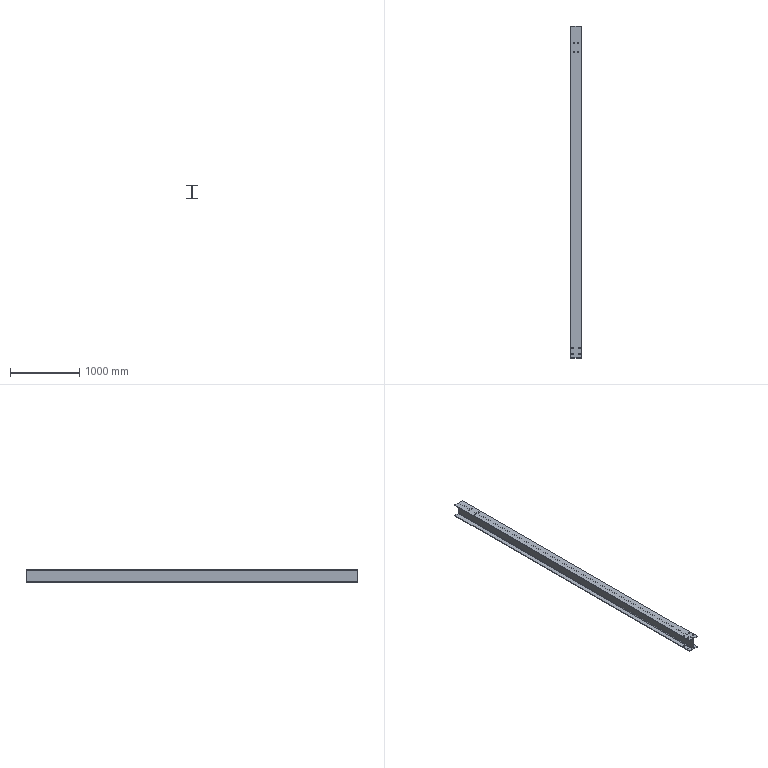Part | STEP file | 中转釜立柱1主体_Default<As Machined> | 1 solid | 42 faces | box 150 x 4780 x 194 mm | volume 18189508 mm3 | cylinder 28 | plane 14 | commonest cylinder face diameters 19 x16 15 x8 16 x4